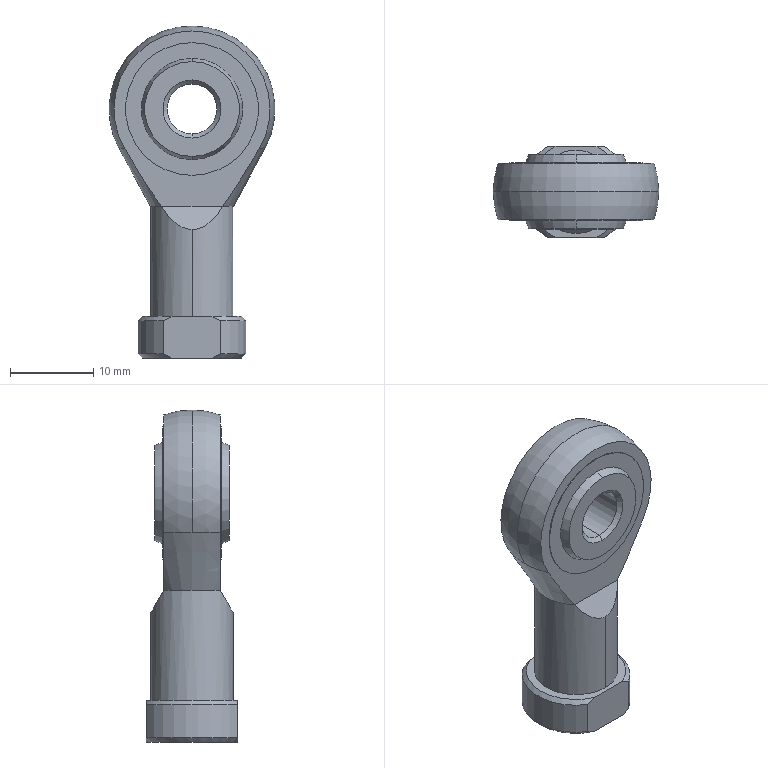Part | STEP file | 001-006-F_M6X100U | 1 solid | 45 faces | box 20 x 11 x 40 mm | volume 3632 mm3 | cone 15 | cylinder 12 | plane 12 | other 4 | sphere 2 | commonest cylinder face diameters 16 x4 4.917 x2 6 x2 10 x2 13 x2